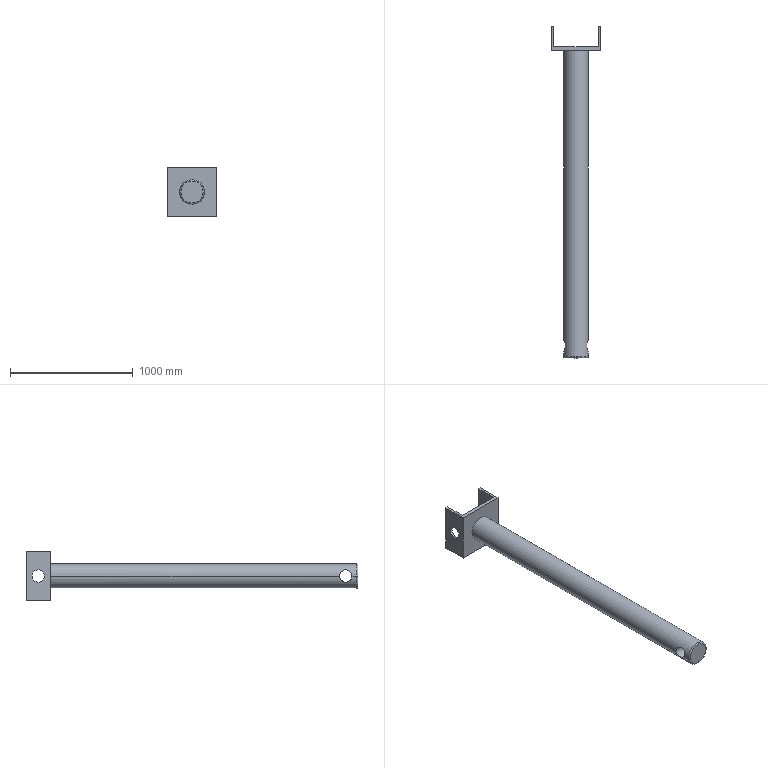Part | SolidWorks | features ICE 3, Extrusion 1, Fillet 1 | 1 solid | 21 faces | box 400 x 2700 x 400 mm | volume 84212442 mm3 | plane 11 | cylinder 8 | torus 2 | commonest cylinder face diameters 100 x6 200 x2
STEP:
#1=CARTESIAN_POINT('',(-100.,-2520.,200.));
#2=VERTEX_POINT('',#1);
#3=CARTESIAN_POINT('',(100.,-2520.,200.));
#4=VERTEX_POINT('',#3);
#5=CARTESIAN_POINT('',(0.,-2520.,200.));
#6=DIRECTION('',(0.,1.,0.));
#7=DIRECTION('',(1.,0.,0.));
#8=AXIS2_PLACEMENT_3D('',#5,#6,#7);
#9=CIRCLE('',#8,100.);
#10=EDGE_CURVE('',#2,#4,#9,.T.);
#11=ORIENTED_EDGE('',*,*,#10,.F.);
#12=CARTESIAN_POINT('',(-90.,-2530.,200.));
#13=VERTEX_POINT('',#12);
#14=CARTESIAN_POINT('',(-90.,-2520.,200.));
#15=DIRECTION('',(0.,0.,1.));
#16=DIRECTION('',(1.,0.,0.));
#17=AXIS2_PLACEMENT_3D('',#14,#15,#16);
#18=CIRCLE('',#17,10.);
#19=EDGE_CURVE('',#2,#13,#18,.T.);
#20=ORIENTED_EDGE('',*,*,#19,.T.);
#21=CARTESIAN_POINT('',(90.,-2530.,200.));
#22=VERTEX_POINT('',#21);
#23=CARTESIAN_POINT('',(0.,-2530.,200.));
#24=DIRECTION('',(0.,-1.,0.));
#25=DIRECTION('',(1.,0.,0.));
#26=AXIS2_PLACEMENT_3D('',#23,#24,#25);
#27=CIRCLE('',#26,90.);
#28=EDGE_CURVE('',#22,#13,#27,.T.);
#29=ORIENTED_EDGE('',*,*,#28,.F.);
#30=CARTESIAN_POINT('',(90.,-2520.,200.));
#31=DIRECTION('',(0.,0.,-1.));
#32=DIRECTION('',(-1.,0.,0.));
#33=AXIS2_PLACEMENT_3D('',#30,#31,#32);
#34=CIRCLE('',#33,10.);
#35=EDGE_CURVE('',#4,#22,#34,.T.);
#36=ORIENTED_EDGE('',*,*,#35,.F.);
#37=EDGE_LOOP('',(#11,#20,#29,#36));
#38=FACE_OUTER_BOUND('',#37,.T.);
#39=CARTESIAN_POINT('',(0.,-2520.,200.));
#40=DIRECTION('',(0.,-1.,0.));
#41=DIRECTION('',(1.,0.,0.));
#42=AXIS2_PLACEMENT_3D('',#39,#40,#41);
#43=TOROIDAL_SURFACE('',#42,90.,10.);
#44=ADVANCED_FACE('',(#38),#43,.T.);
#45=CARTESIAN_POINT('',(100.,-2480.,200.));
#46=VERTEX_POINT('',#45);
#47=CARTESIAN_POINT('',(86.603,-2430.,150.));
#48=VERTEX_POINT('',#47);
#49=CARTESIAN_POINT('',(100.,-2480.,200.));
#50=CARTESIAN_POINT('',(100.,-2480.,199.167));
#51=CARTESIAN_POINT('',(99.99,-2479.979,198.332));
#52=CARTESIAN_POINT('',(99.948,-2479.895,196.655));
#53=CARTESIAN_POINT('',(99.916,-2479.832,195.817));
#54=CARTESIAN_POINT('',(99.791,-2479.581,193.326));
#55=CARTESIAN_POINT('',(99.667,-2479.332,191.687));
#56=CARTESIAN_POINT('',(99.344,-2478.676,188.45));
#57=CARTESIAN_POINT('',(99.145,-2478.269,186.853));
#58=CARTESIAN_POINT('',(98.793,-2477.54,184.487));
#59=CARTESIAN_POINT('',(98.666,-2477.277,183.704));
#60=CARTESIAN_POINT('',(98.397,-2476.712,182.148));
#61=CARTESIAN_POINT('',(98.253,-2476.409,181.376));
#62=CARTESIAN_POINT('',(97.504,-2474.814,177.583));
#63=CARTESIAN_POINT('',(96.795,-2473.266,174.73));
#64=CARTESIAN_POINT('',(95.817,-2471.002,171.373));
#65=CARTESIAN_POINT('',(95.617,-2470.532,170.712));
#66=CARTESIAN_POINT('',(95.209,-2469.559,169.411));
#67=CARTESIAN_POINT('',(95.001,-2469.055,168.77));
#68=CARTESIAN_POINT('',(94.371,-2467.507,166.896));
#69=CARTESIAN_POINT('',(93.944,-2466.422,165.707));
#70=CARTESIAN_POINT('',(92.657,-2463.013,162.311));
#71=CARTESIAN_POINT('',(91.792,-2460.535,160.274));
#72=CARTESIAN_POINT('',(90.759,-2457.159,158.012));
#73=CARTESIAN_POINT('',(90.555,-2456.471,157.574));
#74=CARTESIAN_POINT('',(90.159,-2455.08,156.738));
#75=CARTESIAN_POINT('',(89.965,-2454.377,156.337));
#76=CARTESIAN_POINT('',(89.402,-2452.239,155.189));
#77=CARTESIAN_POINT('',(89.049,-2450.779,154.493));
#78=CARTESIAN_POINT('',(88.398,-2447.788,153.243));
#79=CARTESIAN_POINT('',(88.102,-2446.257,152.688));
#80=CARTESIAN_POINT('',(87.708,-2443.902,151.965));
#81=CARTESIAN_POINT('',(87.585,-2443.108,151.742));
#82=CARTESIAN_POINT('',(87.359,-2441.499,151.333));
#83=CARTESIAN_POINT('',(87.255,-2440.683,151.147));
#84=CARTESIAN_POINT('',(86.793,-2436.603,150.326));
#85=CARTESIAN_POINT('',(86.603,-2433.314,150.));
#86=CARTESIAN_POINT('',(86.603,-2430.,150.));
#87=B_SPLINE_CURVE_WITH_KNOTS('',3,(#49,#50,#51,#52,#53,#54,#55,#56,#57,#58,#59,#60,#61,#62,#63,#64,#65,#66,#67,#68,#69,#70,#71,#72,#73,#74,#75,#76,#77,#78,#79,#80,#81,#82,#83,#84,#85,#86),.UNSPECIFIED.,.F.,.F.,(4,2,2,2,2,2,2,2,2,2,2,2,2,2,2,2,2,2,4),(0.07955,0.08203,0.08452,0.08948,0.09445,0.09693,0.09942,0.1094,0.1118,0.1143,0.1193,0.1292,0.1317,0.1342,0.1392,0.1441,0.1466,0.1491,0.159),.UNSPECIFIED.);
#88=EDGE_CURVE('',#46,#48,#87,.T.);
#89=ORIENTED_EDGE('',*,*,#88,.T.);
#90=CARTESIAN_POINT('',(-86.603,-2430.,150.));
#91=VERTEX_POINT('',#90);
#92=CARTESIAN_POINT('',(2500.,-2430.,150.));
#93=DIRECTION('',(-1.,0.,0.));
#94=VECTOR('',#93,1000.);
#95=LINE('',#92,#94);
#96=EDGE_CURVE('',#48,#91,#95,.T.);
#97=ORIENTED_EDGE('',*,*,#96,.T.);
#98=CARTESIAN_POINT('',(-100.,-2480.,200.));
#99=VERTEX_POINT('',#98);
#100=CARTESIAN_POINT('',(-86.603,-2430.,150.));
#101=CARTESIAN_POINT('',(-86.603,-2431.652,150.));
#102=CARTESIAN_POINT('',(-86.65,-2433.306,150.082));
#103=CARTESIAN_POINT('',(-86.792,-2435.79,150.329));
#104=CARTESIAN_POINT('',(-86.851,-2436.618,150.433));
#105=CARTESIAN_POINT('',(-86.993,-2438.274,150.682));
#106=CARTESIAN_POINT('',(-87.075,-2439.095,150.827));
#107=CARTESIAN_POINT('',(-87.537,-2443.158,151.648));
#108=CARTESIAN_POINT('',(-88.072,-2446.288,152.614));
#109=CARTESIAN_POINT('',(-88.893,-2450.064,154.195));
#110=CARTESIAN_POINT('',(-89.066,-2450.813,154.53));
#111=CARTESIAN_POINT('',(-89.423,-2452.292,155.237));
#112=CARTESIAN_POINT('',(-89.607,-2453.019,155.607));
#113=CARTESIAN_POINT('',(-90.174,-2455.164,156.763));
#114=CARTESIAN_POINT('',(-90.571,-2456.545,157.598));
#115=CARTESIAN_POINT('',(-91.389,-2459.216,159.392));
#116=CARTESIAN_POINT('',(-91.811,-2460.506,160.352));
#117=CARTESIAN_POINT('',(-92.454,-2462.374,161.887));
#118=CARTESIAN_POINT('',(-92.67,-2462.985,162.415));
#119=CARTESIAN_POINT('',(-93.104,-2464.185,163.503));
#120=CARTESIAN_POINT('',(-93.321,-2464.771,164.061));
#121=CARTESIAN_POINT('',(-94.398,-2467.622,166.91));
#122=CARTESIAN_POINT('',(-95.238,-2469.661,169.382));
#123=CARTESIAN_POINT('',(-96.406,-2472.364,173.394));
#124=CARTESIAN_POINT('',(-96.779,-2473.205,174.781));
#125=CARTESIAN_POINT('',(-97.309,-2474.375,176.945));
#126=CARTESIAN_POINT('',(-97.48,-2474.748,177.677));
#127=CARTESIAN_POINT('',(-97.806,-2475.454,179.153));
#128=CARTESIAN_POINT('',(-97.962,-2475.789,179.899));
#129=CARTESIAN_POINT('',(-98.704,-2477.367,183.66));
#130=CARTESIAN_POINT('',(-99.176,-2478.335,186.782));
#131=CARTESIAN_POINT('',(-99.583,-2479.16,190.837));
#132=CARTESIAN_POINT('',(-99.655,-2479.306,191.655));
#133=CARTESIAN_POINT('',(-99.779,-2479.557,193.308));
#134=CARTESIAN_POINT('',(-99.832,-2479.663,194.142));
#135=CARTESIAN_POINT('',(-99.916,-2479.831,195.81));
#136=CARTESIAN_POINT('',(-99.947,-2479.894,196.645));
#137=CARTESIAN_POINT('',(-99.989,-2479.979,198.32));
#138=CARTESIAN_POINT('',(-100.,-2480.,199.161));
#139=CARTESIAN_POINT('',(-100.,-2480.,200.));
#140=B_SPLINE_CURVE_WITH_KNOTS('',3,(#100,#101,#102,#103,#104,#105,#106,#107,#108,#109,#110,#111,#112,#113,#114,#115,#116,#117,#118,#119,#120,#121,#122,#123,#124,#125,#126,#127,#128,#129,#130,#131,#132,#133,#134,#135,#136,#137,#138,#139),.UNSPECIFIED.,.F.,.F.,(4,2,2,2,2,2,2,2,2,2,2,2,2,2,2,2,2,2,2,4),(0.2385,0.2434,0.2459,0.2484,0.2583,0.2608,0.2633,0.2682,0.2732,0.2757,0.2782,0.2881,0.293,0.2955,0.298,0.3079,0.3104,0.3129,0.3153,0.3178),.UNSPECIFIED.);
#141=EDGE_CURVE('',#91,#99,#140,.T.);
#142=ORIENTED_EDGE('',*,*,#141,.T.);
#143=CARTESIAN_POINT('',(-86.603,-2430.,250.));
#144=VERTEX_POINT('',#143);
#145=CARTESIAN_POINT('',(-100.,-2480.,200.));
#146=CARTESIAN_POINT('',(-100.,-2480.,203.367));
#147=CARTESIAN_POINT('',(-99.831,-2479.663,206.667));
#148=CARTESIAN_POINT('',(-99.347,-2478.682,211.524));
#149=CARTESIAN_POINT('',(-99.148,-2478.275,213.128));
#150=CARTESIAN_POINT('',(-98.793,-2477.541,215.509));
#151=CARTESIAN_POINT('',(-98.666,-2477.276,216.298));
#152=CARTESIAN_POINT('',(-98.397,-2476.712,217.851));
#153=CARTESIAN_POINT('',(-98.255,-2476.412,218.617));
#154=CARTESIAN_POINT('',(-97.509,-2474.825,222.392));
#155=CARTESIAN_POINT('',(-96.801,-2473.28,225.247));
#156=CARTESIAN_POINT('',(-95.819,-2471.006,228.621));
#157=CARTESIAN_POINT('',(-95.618,-2470.533,229.287));
#158=CARTESIAN_POINT('',(-95.209,-2469.559,230.589));
#159=CARTESIAN_POINT('',(-95.002,-2469.059,231.226));
#160=CARTESIAN_POINT('',(-94.375,-2467.517,233.092));
#161=CARTESIAN_POINT('',(-93.949,-2466.435,234.279));
#162=CARTESIAN_POINT('',(-93.091,-2464.163,236.544));
#163=CARTESIAN_POINT('',(-92.66,-2462.973,237.622));
#164=CARTESIAN_POINT('',(-92.017,-2461.104,239.156));
#165=CARTESIAN_POINT('',(-91.803,-2460.467,239.654));
#166=CARTESIAN_POINT('',(-91.379,-2459.164,240.621));
#167=CARTESIAN_POINT('',(-91.169,-2458.499,241.091));
#168=CARTESIAN_POINT('',(-90.139,-2455.133,243.345));
#169=CARTESIAN_POINT('',(-89.378,-2452.293,244.873));
#170=CARTESIAN_POINT('',(-88.4,-2447.797,246.754));
#171=CARTESIAN_POINT('',(-88.102,-2446.258,247.312));
#172=CARTESIAN_POINT('',(-87.705,-2443.886,248.04));
#173=CARTESIAN_POINT('',(-87.581,-2443.082,248.265));
#174=CARTESIAN_POINT('',(-87.356,-2441.473,248.673));
#175=CARTESIAN_POINT('',(-87.253,-2440.665,248.856));
#176=CARTESIAN_POINT('',(-86.795,-2436.615,249.671));
#177=CARTESIAN_POINT('',(-86.603,-2433.33,250.));
#178=CARTESIAN_POINT('',(-86.603,-2430.,250.));
#179=B_SPLINE_CURVE_WITH_KNOTS('',3,(#145,#146,#147,#148,#149,#150,#151,#152,#153,#154,#155,#156,#157,#158,#159,#160,#161,#162,#163,#164,#165,#166,#167,#168,#169,#170,#171,#172,#173,#174,#175,#176,#177,#178),.UNSPECIFIED.,.F.,.F.,(4,2,2,2,2,2,2,2,2,2,2,2,2,2,2,2,4),(0.,0.009947,0.01492,0.01741,0.01989,0.02984,0.03233,0.03481,0.03979,0.04476,0.04725,0.04973,0.05968,0.06465,0.06714,0.06963,0.07957),.UNSPECIFIED.);
#180=EDGE_CURVE('',#99,#144,#179,.T.);
#181=ORIENTED_EDGE('',*,*,#180,.T.);
#182=CARTESIAN_POINT('',(86.603,-2430.,250.));
#183=VERTEX_POINT('',#182);
#184=CARTESIAN_POINT('',(2500.,-2430.,250.));
#185=DIRECTION('',(-1.,0.,0.));
#186=VECTOR('',#185,1000.);
#187=LINE('',#184,#186);
#188=EDGE_CURVE('',#183,#144,#187,.T.);
#189=ORIENTED_EDGE('',*,*,#188,.F.);
#190=CARTESIAN_POINT('',(86.603,-2430.,250.));
#191=CARTESIAN_POINT('',(86.603,-2433.368,250.));
#192=CARTESIAN_POINT('',(86.799,-2436.665,249.663));
#193=CARTESIAN_POINT('',(87.35,-2441.515,248.684));
#194=CARTESIAN_POINT('',(87.576,-2443.115,248.278));
#195=CARTESIAN_POINT('',(87.974,-2445.491,247.547));
#196=CARTESIAN_POINT('',(88.116,-2446.278,247.283));
#197=CARTESIAN_POINT('',(88.415,-2447.825,246.722));
#198=CARTESIAN_POINT('',(88.572,-2448.589,246.423));
#199=CARTESIAN_POINT('',(89.392,-2452.352,244.845));
#200=CARTESIAN_POINT('',(90.158,-2455.199,243.308));
#201=CARTESIAN_POINT('',(91.19,-2458.567,241.044));
#202=CARTESIAN_POINT('',(91.401,-2459.232,240.573));
#203=CARTESIAN_POINT('',(91.825,-2460.531,239.604));
#204=CARTESIAN_POINT('',(92.038,-2461.167,239.106));
#205=CARTESIAN_POINT('',(92.681,-2463.031,237.571));
#206=CARTESIAN_POINT('',(93.112,-2464.219,236.492));
#207=CARTESIAN_POINT('',(93.969,-2466.486,234.224));
#208=CARTESIAN_POINT('',(94.395,-2467.567,233.035));
#209=CARTESIAN_POINT('',(95.022,-2469.107,231.166));
#210=CARTESIAN_POINT('',(95.229,-2469.607,230.528));
#211=CARTESIAN_POINT('',(95.637,-2470.579,229.223));
#212=CARTESIAN_POINT('',(95.838,-2471.051,228.557));
#213=CARTESIAN_POINT('',(96.817,-2473.316,225.186));
#214=CARTESIAN_POINT('',(97.521,-2474.852,222.338));
#215=CARTESIAN_POINT('',(98.41,-2476.742,217.828));
#216=CARTESIAN_POINT('',(98.678,-2477.303,216.285));
#217=CARTESIAN_POINT('',(99.032,-2478.034,213.906));
#218=CARTESIAN_POINT('',(99.141,-2478.26,213.101));
#219=CARTESIAN_POINT('',(99.341,-2478.669,211.489));
#220=CARTESIAN_POINT('',(99.431,-2478.853,210.68));
#221=CARTESIAN_POINT('',(99.834,-2479.67,206.623));
#222=CARTESIAN_POINT('',(100.,-2480.,203.334));
#223=CARTESIAN_POINT('',(100.,-2480.,200.));
#224=B_SPLINE_CURVE_WITH_KNOTS('',3,(#190,#191,#192,#193,#194,#195,#196,#197,#198,#199,#200,#201,#202,#203,#204,#205,#206,#207,#208,#209,#210,#211,#212,#213,#214,#215,#216,#217,#218,#219,#220,#221,#222,#223),.UNSPECIFIED.,.F.,.F.,(4,2,2,2,2,2,2,2,2,2,2,2,2,2,2,2,4),(0.,0.009943,0.01492,0.0174,0.01989,0.02983,0.03232,0.0348,0.03977,0.04475,0.04723,0.04972,0.05966,0.06463,0.06712,0.0696,0.07955),.UNSPECIFIED.);
#225=EDGE_CURVE('',#183,#46,#224,.T.);
#226=ORIENTED_EDGE('',*,*,#225,.T.);
#227=EDGE_LOOP('',(#89,#97,#142,#181,#189,#226));
#228=FACE_OUTER_BOUND('',#227,.T.);
#229=CARTESIAN_POINT('',(2500.,-2430.,200.));
#230=DIRECTION('',(-1.,0.,0.));
#231=DIRECTION('',(0.,0.,1.));
#232=AXIS2_PLACEMENT_3D('',#229,#230,#231);
#233=CYLINDRICAL_SURFACE('',#232,50.);
#234=ADVANCED_FACE('',(#228),#233,.F.);
#235=CARTESIAN_POINT('',(-200.,20.,200.));
#236=VERTEX_POINT('',#235);
#237=CARTESIAN_POINT('',(-200.,120.,200.));
#238=VERTEX_POINT('',#237);
#239=CARTESIAN_POINT('',(-200.,70.,200.));
#240=DIRECTION('',(1.,0.,0.));
#241=DIRECTION('',(0.,1.,0.));
#242=AXIS2_PLACEMENT_3D('',#239,#240,#241);
#243=CIRCLE('',#242,50.);
#244=EDGE_CURVE('',#236,#238,#243,.T.);
#245=ORIENTED_EDGE('',*,*,#244,.F.);
#246=CARTESIAN_POINT('',(-180.,20.,200.));
#247=VERTEX_POINT('',#246);
#248=CARTESIAN_POINT('',(-200.,20.,200.));
#249=DIRECTION('',(1.,0.,0.));
#250=VECTOR('',#249,1000.);
#251=LINE('',#248,#250);
#252=EDGE_CURVE('',#236,#247,#251,.T.);
#253=ORIENTED_EDGE('',*,*,#252,.T.);
#254=CARTESIAN_POINT('',(-180.,120.,200.));
#255=VERTEX_POINT('',#254);
#256=CARTESIAN_POINT('',(-180.,70.,200.));
#257=DIRECTION('',(-1.,0.,0.));
#258=DIRECTION('',(0.,-1.,0.));
#259=AXIS2_PLACEMENT_3D('',#256,#257,#258);
#260=CIRCLE('',#259,50.);
#261=EDGE_CURVE('',#255,#247,#260,.T.);
#262=ORIENTED_EDGE('',*,*,#261,.F.);
#263=CARTESIAN_POINT('',(-200.,120.,200.));
#264=DIRECTION('',(1.,0.,0.));
#265=VECTOR('',#264,1000.);
#266=LINE('',#263,#265);
#267=EDGE_CURVE('',#238,#255,#266,.T.);
#268=ORIENTED_EDGE('',*,*,#267,.F.);
#269=EDGE_LOOP('',(#245,#253,#262,#268));
#270=FACE_OUTER_BOUND('',#269,.T.);
#271=CARTESIAN_POINT('',(-200.,70.,200.));
#272=DIRECTION('',(1.,0.,0.));
#273=DIRECTION('',(0.,1.,0.));
#274=AXIS2_PLACEMENT_3D('',#271,#272,#273);
#275=CYLINDRICAL_SURFACE('',#274,50.);
#276=ADVANCED_FACE('',(#270),#275,.F.);
#277=CARTESIAN_POINT('',(180.,20.,200.));
#278=VERTEX_POINT('',#277);
#279=CARTESIAN_POINT('',(180.,120.,200.));
#280=VERTEX_POINT('',#279);
#281=CARTESIAN_POINT('',(180.,70.,200.));
#282=DIRECTION('',(1.,0.,0.));
#283=DIRECTION('',(0.,0.,-1.));
#284=AXIS2_PLACEMENT_3D('',#281,#282,#283);
#285=CIRCLE('',#284,50.);
#286=EDGE_CURVE('',#278,#280,#285,.T.);
#287=ORIENTED_EDGE('',*,*,#286,.F.);
#288=CARTESIAN_POINT('',(200.,20.,200.));
#289=VERTEX_POINT('',#288);
#290=CARTESIAN_POINT('',(-200.,20.,200.));
#291=DIRECTION('',(1.,0.,0.));
#292=VECTOR('',#291,1000.);
#293=LINE('',#290,#292);
#294=EDGE_CURVE('',#278,#289,#293,.T.);
#295=ORIENTED_EDGE('',*,*,#294,.T.);
#296=CARTESIAN_POINT('',(200.,120.,200.));
#297=VERTEX_POINT('',#296);
#298=CARTESIAN_POINT('',(200.,70.,200.));
#299=DIRECTION('',(1.,0.,0.));
#300=DIRECTION('',(0.,1.,0.));
#301=AXIS2_PLACEMENT_3D('',#298,#299,#300);
#302=CIRCLE('',#301,50.);
#303=EDGE_CURVE('',#289,#297,#302,.T.);
#304=ORIENTED_EDGE('',*,*,#303,.T.);
#305=CARTESIAN_POINT('',(-200.,120.,200.));
#306=DIRECTION('',(1.,0.,0.));
#307=VECTOR('',#306,1000.);
#308=LINE('',#305,#307);
#309=EDGE_CURVE('',#280,#297,#308,.T.);
#310=ORIENTED_EDGE('',*,*,#309,.F.);
#311=EDGE_LOOP('',(#287,#295,#304,#310));
#312=FACE_OUTER_BOUND('',#311,.T.);
#313=CARTESIAN_POINT('',(-200.,70.,200.));
#314=DIRECTION('',(1.,0.,0.));
#315=DIRECTION('',(0.,1.,0.));
#316=AXIS2_PLACEMENT_3D('',#313,#314,#315);
#317=CYLINDRICAL_SURFACE('',#316,50.);
#318=ADVANCED_FACE('',(#312),#317,.F.);
#319=ORIENTED_EDGE('',*,*,#10,.T.);
#320=CARTESIAN_POINT('',(100.,-2530.,200.));
#321=DIRECTION('',(0.,1.,0.));
#322=VECTOR('',#321,1000.);
#323=LINE('',#320,#322);
#324=EDGE_CURVE('',#4,#46,#323,.T.);
#325=ORIENTED_EDGE('',*,*,#324,.T.);
#326=ORIENTED_EDGE('',*,*,#225,.F.);
#327=CARTESIAN_POINT('',(100.,-2380.,200.));
#328=VERTEX_POINT('',#327);
#329=CARTESIAN_POINT('',(100.,-2380.,200.));
#330=CARTESIAN_POINT('',(100.,-2380.,201.654));
#331=CARTESIAN_POINT('',(99.959,-2380.082,203.31));
#332=CARTESIAN_POINT('',(99.835,-2380.33,205.797));
#333=CARTESIAN_POINT('',(99.784,-2380.434,206.628));
#334=CARTESIAN_POINT('',(99.66,-2380.684,208.284));
#335=CARTESIAN_POINT('',(99.588,-2380.829,209.104));
#336=CARTESIAN_POINT('',(99.183,-2381.652,213.17));
#337=CARTESIAN_POINT('',(98.71,-2382.62,216.308));
#338=CARTESIAN_POINT('',(97.964,-2384.208,220.093));
#339=CARTESIAN_POINT('',(97.806,-2384.545,220.844));
#340=CARTESIAN_POINT('',(97.478,-2385.255,222.329));
#341=CARTESIAN_POINT('',(97.308,-2385.627,223.059));
#342=CARTESIAN_POINT('',(96.781,-2386.79,225.211));
#343=CARTESIAN_POINT('',(96.408,-2387.63,226.596));
#344=CARTESIAN_POINT('',(95.63,-2389.432,229.272));
#345=CARTESIAN_POINT('',(95.224,-2390.396,230.563));
#346=CARTESIAN_POINT('',(94.598,-2391.935,232.43));
#347=CARTESIAN_POINT('',(94.386,-2392.464,233.041));
#348=CARTESIAN_POINT('',(93.958,-2393.554,234.24));
#349=CARTESIAN_POINT('',(93.741,-2394.115,234.827));
#350=CARTESIAN_POINT('',(92.663,-2396.97,237.676));
#351=CARTESIAN_POINT('',(91.8,-2399.444,239.707));
#352=CARTESIAN_POINT('',(90.573,-2403.448,242.398));
#353=CARTESIAN_POINT('',(90.175,-2404.832,243.235));
#354=CARTESIAN_POINT('',(89.605,-2406.988,244.397));
#355=CARTESIAN_POINT('',(89.42,-2407.718,244.768));
#356=CARTESIAN_POINT('',(89.065,-2409.19,245.471));
#357=CARTESIAN_POINT('',(88.894,-2409.932,245.803));
#358=CARTESIAN_POINT('',(88.078,-2413.681,247.374));
#359=CARTESIAN_POINT('',(87.545,-2416.794,248.337));
#360=CARTESIAN_POINT('',(87.082,-2420.839,249.161));
#361=CARTESIAN_POINT('',(87.,-2421.656,249.306));
#362=CARTESIAN_POINT('',(86.857,-2423.306,249.557));
#363=CARTESIAN_POINT('',(86.797,-2424.14,249.663));
#364=CARTESIAN_POINT('',(86.7,-2425.808,249.831));
#365=CARTESIAN_POINT('',(86.663,-2426.644,249.894));
#366=CARTESIAN_POINT('',(86.615,-2428.319,249.979));
#367=CARTESIAN_POINT('',(86.603,-2429.16,250.));
#368=CARTESIAN_POINT('',(86.603,-2430.,250.));
#369=B_SPLINE_CURVE_WITH_KNOTS('',3,(#329,#330,#331,#332,#333,#334,#335,#336,#337,#338,#339,#340,#341,#342,#343,#344,#345,#346,#347,#348,#349,#350,#351,#352,#353,#354,#355,#356,#357,#358,#359,#360,#361,#362,#363,#364,#365,#366,#367,#368),.UNSPECIFIED.,.F.,.F.,(4,2,2,2,2,2,2,2,2,2,2,2,2,2,2,2,2,2,2,4),(0.2384,0.2434,0.2459,0.2484,0.2583,0.2608,0.2632,0.2682,0.2732,0.2756,0.2781,0.288,0.293,0.2955,0.2979,0.3079,0.3103,0.3128,0.3153,0.3178),.UNSPECIFIED.);
#370=EDGE_CURVE('',#328,#183,#369,.T.);
#371=ORIENTED_EDGE('',*,*,#370,.F.);
#372=CARTESIAN_POINT('',(100.,-30.,200.));
#373=VERTEX_POINT('',#372);
#374=CARTESIAN_POINT('',(100.,-2530.,200.));
#375=DIRECTION('',(0.,1.,0.));
#376=VECTOR('',#375,1000.);
#377=LINE('',#374,#376);
#378=EDGE_CURVE('',#328,#373,#377,.T.);
#379=ORIENTED_EDGE('',*,*,#378,.T.);
#380=CARTESIAN_POINT('',(-100.,-30.,200.));
#381=VERTEX_POINT('',#380);
#382=CARTESIAN_POINT('',(0.,-30.,200.));
#383=DIRECTION('',(0.,-1.,0.));
#384=DIRECTION('',(-1.,0.,0.));
#385=AXIS2_PLACEMENT_3D('',#382,#383,#384);
#386=CIRCLE('',#385,100.);
#387=EDGE_CURVE('',#373,#381,#386,.T.);
#388=ORIENTED_EDGE('',*,*,#387,.T.);
#389=CARTESIAN_POINT('',(-100.,-2380.,200.));
#390=VERTEX_POINT('',#389);
#391=CARTESIAN_POINT('',(-100.,-2530.,200.));
#392=DIRECTION('',(0.,1.,0.));
#393=VECTOR('',#392,1000.);
#394=LINE('',#391,#393);
#395=EDGE_CURVE('',#390,#381,#394,.T.);
#396=ORIENTED_EDGE('',*,*,#395,.F.);
#397=CARTESIAN_POINT('',(-86.603,-2430.,250.));
#398=CARTESIAN_POINT('',(-86.603,-2429.168,250.));
#399=CARTESIAN_POINT('',(-86.615,-2428.334,249.979));
#400=CARTESIAN_POINT('',(-86.663,-2426.66,249.895));
#401=CARTESIAN_POINT('',(-86.699,-2425.82,249.832));
#402=CARTESIAN_POINT('',(-86.843,-2423.328,249.581));
#403=CARTESIAN_POINT('',(-86.986,-2421.689,249.332));
#404=CARTESIAN_POINT('',(-87.354,-2418.457,248.677));
#405=CARTESIAN_POINT('',(-87.58,-2416.862,248.271));
#406=CARTESIAN_POINT('',(-87.975,-2414.502,247.545));
#407=CARTESIAN_POINT('',(-88.116,-2413.721,247.283));
#408=CARTESIAN_POINT('',(-88.416,-2412.169,246.72));
#409=CARTESIAN_POINT('',(-88.574,-2411.4,246.419));
#410=CARTESIAN_POINT('',(-89.399,-2407.621,244.832));
#411=CARTESIAN_POINT('',(-90.165,-2404.776,243.292));
#412=CARTESIAN_POINT('',(-91.193,-2401.424,241.037));
#413=CARTESIAN_POINT('',(-91.402,-2400.764,240.57));
#414=CARTESIAN_POINT('',(-91.826,-2399.464,239.6));
#415=CARTESIAN_POINT('',(-92.041,-2398.824,239.099));
#416=CARTESIAN_POINT('',(-92.686,-2396.953,237.557));
#417=CARTESIAN_POINT('',(-93.118,-2395.765,236.476));
#418=CARTESIAN_POINT('',(-94.403,-2392.365,233.074));
#419=CARTESIAN_POINT('',(-95.246,-2390.32,230.596));
#420=CARTESIAN_POINT('',(-96.229,-2388.046,227.212));
#421=CARTESIAN_POINT('',(-96.421,-2387.606,226.523));
#422=CARTESIAN_POINT('',(-96.794,-2386.766,225.129));
#423=CARTESIAN_POINT('',(-96.974,-2386.363,224.423));
#424=CARTESIAN_POINT('',(-97.498,-2385.209,222.28));
#425=CARTESIAN_POINT('',(-97.822,-2384.51,220.816));
#426=CARTESIAN_POINT('',(-98.412,-2383.253,217.815));
#427=CARTESIAN_POINT('',(-98.679,-2382.696,216.279));
#428=CARTESIAN_POINT('',(-99.03,-2381.969,213.919));
#429=CARTESIAN_POINT('',(-99.139,-2381.745,213.122));
#430=CARTESIAN_POINT('',(-99.339,-2381.336,211.51));
#431=CARTESIAN_POINT('',(-99.43,-2381.15,210.692));
#432=CARTESIAN_POINT('',(-99.835,-2380.327,206.61));
#433=CARTESIAN_POINT('',(-100.,-2380.,203.318));
#434=CARTESIAN_POINT('',(-100.,-2380.,200.));
#435=B_SPLINE_CURVE_WITH_KNOTS('',3,(#397,#398,#399,#400,#401,#402,#403,#404,#405,#406,#407,#408,#409,#410,#411,#412,#413,#414,#415,#416,#417,#418,#419,#420,#421,#422,#423,#424,#425,#426,#427,#428,#429,#430,#431,#432,#433,#434),.UNSPECIFIED.,.F.,.F.,(4,2,2,2,2,2,2,2,2,2,2,2,2,2,2,2,2,2,4),(0.07957,0.08206,0.08454,0.08951,0.09447,0.09696,0.09944,0.1094,0.1119,0.1143,0.1193,0.1292,0.1317,0.1342,0.1392,0.1441,0.1466,0.1491,0.159),.UNSPECIFIED.);
#436=EDGE_CURVE('',#144,#390,#435,.T.);
#437=ORIENTED_EDGE('',*,*,#436,.F.);
#438=ORIENTED_EDGE('',*,*,#180,.F.);
#439=CARTESIAN_POINT('',(-100.,-2530.,200.));
#440=DIRECTION('',(0.,1.,0.));
#441=VECTOR('',#440,1000.);
#442=LINE('',#439,#441);
#443=EDGE_CURVE('',#2,#99,#442,.T.);
#444=ORIENTED_EDGE('',*,*,#443,.F.);
#445=EDGE_LOOP('',(#319,#325,#326,#371,#379,#388,#396,#437,#438,#444));
#446=FACE_OUTER_BOUND('',#445,.T.);
#447=CARTESIAN_POINT('',(0.,-2530.,200.));
#448=DIRECTION('',(0.,1.,0.));
#449=DIRECTION('',(-1.,0.,0.));
#450=AXIS2_PLACEMENT_3D('',#447,#448,#449);
#451=CYLINDRICAL_SURFACE('',#450,100.);
#452=ADVANCED_FACE('',(#446),#451,.T.);
#453=ORIENTED_EDGE('',*,*,#324,.F.);
#454=CARTESIAN_POINT('',(0.,-2520.,200.));
#455=DIRECTION('',(0.,1.,0.));
#456=DIRECTION('',(1.,0.,0.));
#457=AXIS2_PLACEMENT_3D('',#454,#455,#456);
#458=CIRCLE('',#457,100.);
#459=EDGE_CURVE('',#4,#2,#458,.T.);
#460=ORIENTED_EDGE('',*,*,#459,.T.);
#461=ORIENTED_EDGE('',*,*,#443,.T.);
#462=ORIENTED_EDGE('',*,*,#141,.F.);
#463=CARTESIAN_POINT('',(-100.,-2380.,200.));
#464=CARTESIAN_POINT('',(-100.,-2380.,198.342));
#465=CARTESIAN_POINT('',(-99.959,-2380.082,196.677));
#466=CARTESIAN_POINT('',(-99.792,-2380.418,193.334));
#467=CARTESIAN_POINT('',(-99.667,-2380.668,191.688));
#468=CARTESIAN_POINT('',(-99.182,-2381.654,186.824));
#469=CARTESIAN_POINT('',(-98.708,-2382.623,183.681));
#470=CARTESIAN_POINT('',(-97.956,-2384.223,179.872));
#471=CARTESIAN_POINT('',(-97.799,-2384.561,179.12));
#472=CARTESIAN_POINT('',(-97.472,-2385.269,177.643));
#473=CARTESIAN_POINT('',(-97.302,-2385.64,176.916));
#474=CARTESIAN_POINT('',(-96.776,-2386.801,174.771));
#475=CARTESIAN_POINT('',(-96.404,-2387.64,173.387));
#476=CARTESIAN_POINT('',(-95.624,-2389.447,170.707));
#477=CARTESIAN_POINT('',(-95.216,-2390.414,169.412));
#478=CARTESIAN_POINT('',(-94.586,-2391.964,167.536));
#479=CARTESIAN_POINT('',(-94.373,-2392.497,166.921));
#480=CARTESIAN_POINT('',(-93.945,-2393.586,165.726));
#481=CARTESIAN_POINT('',(-93.731,-2394.143,165.144));
#482=CARTESIAN_POINT('',(-92.656,-2396.99,162.308));
#483=CARTESIAN_POINT('',(-91.792,-2399.465,160.275));
#484=CARTESIAN_POINT('',(-90.765,-2402.82,158.025));
#485=CARTESIAN_POINT('',(-90.563,-2403.504,157.59));
#486=CARTESIAN_POINT('',(-90.164,-2404.9,156.749));
#487=CARTESIAN_POINT('',(-89.969,-2405.61,156.345));
#488=CARTESIAN_POINT('',(-89.402,-2407.759,155.19));
#489=CARTESIAN_POINT('',(-89.048,-2409.223,154.492));
#490=CARTESIAN_POINT('',(-88.073,-2413.712,152.616));
#491=CARTESIAN_POINT('',(-87.538,-2416.832,151.65));
#492=CARTESIAN_POINT('',(-87.074,-2420.913,150.826));
#493=CARTESIAN_POINT('',(-86.992,-2421.74,150.68));
#494=CARTESIAN_POINT('',(-86.851,-2423.39,150.432));
#495=CARTESIAN_POINT('',(-86.792,-2424.215,150.329));
#496=CARTESIAN_POINT('',(-86.65,-2426.692,150.082));
#497=CARTESIAN_POINT('',(-86.603,-2428.345,150.));
#498=CARTESIAN_POINT('',(-86.603,-2430.,150.));
#499=B_SPLINE_CURVE_WITH_KNOTS('',3,(#463,#464,#465,#466,#467,#468,#469,#470,#471,#472,#473,#474,#475,#476,#477,#478,#479,#480,#481,#482,#483,#484,#485,#486,#487,#488,#489,#490,#491,#492,#493,#494,#495,#496,#497,#498),.UNSPECIFIED.,.F.,.F.,(4,2,2,2,2,2,2,2,2,2,2,2,2,2,2,2,2,4),(0.159,0.164,0.169,0.1789,0.1814,0.1839,0.1888,0.1938,0.1963,0.1988,0.2087,0.2112,0.2137,0.2186,0.2286,0.231,0.2335,0.2385),.UNSPECIFIED.);
#500=EDGE_CURVE('',#390,#91,#499,.T.);
#501=ORIENTED_EDGE('',*,*,#500,.F.);
#502=ORIENTED_EDGE('',*,*,#395,.T.);
#503=CARTESIAN_POINT('',(0.,-30.,200.));
#504=DIRECTION('',(0.,-1.,0.));
#505=DIRECTION('',(-1.,0.,0.));
#506=AXIS2_PLACEMENT_3D('',#503,#504,#505);
#507=CIRCLE('',#506,100.);
#508=EDGE_CURVE('',#381,#373,#507,.T.);
#509=ORIENTED_EDGE('',*,*,#508,.T.);
#510=ORIENTED_EDGE('',*,*,#378,.F.);
#511=CARTESIAN_POINT('',(86.603,-2430.,150.));
#512=CARTESIAN_POINT('',(86.603,-2428.344,150.));
#513=CARTESIAN_POINT('',(86.65,-2426.682,150.082));
#514=CARTESIAN_POINT('',(86.794,-2424.179,150.333));
#515=CARTESIAN_POINT('',(86.854,-2423.347,150.438));
#516=CARTESIAN_POINT('',(86.995,-2421.701,150.687));
#517=CARTESIAN_POINT('',(87.077,-2420.884,150.831));
#518=CARTESIAN_POINT('',(87.538,-2416.835,151.651));
#519=CARTESIAN_POINT('',(88.073,-2413.699,152.617));
#520=CARTESIAN_POINT('',(89.067,-2409.142,154.529));
#521=CARTESIAN_POINT('',(89.425,-2407.669,155.234));
#522=CARTESIAN_POINT('',(90.179,-2404.817,156.774));
#523=CARTESIAN_POINT('',(90.576,-2403.437,157.609));
#524=CARTESIAN_POINT('',(91.396,-2400.762,159.408));
#525=CARTESIAN_POINT('',(91.82,-2399.468,160.372));
#526=CARTESIAN_POINT('',(92.466,-2397.591,161.917));
#527=CARTESIAN_POINT('',(92.683,-2396.977,162.448));
#528=CARTESIAN_POINT('',(93.116,-2395.783,163.533));
#529=CARTESIAN_POINT('',(93.331,-2395.2,164.089));
#530=CARTESIAN_POINT('',(94.405,-2392.362,166.929));
#531=CARTESIAN_POINT('',(95.245,-2390.322,169.403));
#532=CARTESIAN_POINT('',(96.222,-2388.061,172.765));
#533=CARTESIAN_POINT('',(96.414,-2387.623,173.451));
#534=CARTESIAN_POINT('',(96.789,-2386.777,174.851));
#535=CARTESIAN_POINT('',(96.971,-2386.371,175.563));
#536=CARTESIAN_POINT('',(97.497,-2385.209,177.719));
#537=CARTESIAN_POINT('',(97.822,-2384.508,179.187));
#538=CARTESIAN_POINT('',(98.709,-2382.623,183.691));
#539=CARTESIAN_POINT('',(99.182,-2381.653,186.821));
#540=CARTESIAN_POINT('',(99.589,-2380.826,190.909));
#541=CARTESIAN_POINT('',(99.661,-2380.68,191.737));
#542=CARTESIAN_POINT('',(99.785,-2380.432,193.387));
#543=CARTESIAN_POINT('',(99.836,-2380.329,194.212));
#544=CARTESIAN_POINT('',(99.959,-2380.082,196.69));
#545=CARTESIAN_POINT('',(100.,-2380.,198.344));
#546=CARTESIAN_POINT('',(100.,-2380.,200.));
#547=B_SPLINE_CURVE_WITH_KNOTS('',3,(#511,#512,#513,#514,#515,#516,#517,#518,#519,#520,#521,#522,#523,#524,#525,#526,#527,#528,#529,#530,#531,#532,#533,#534,#535,#536,#537,#538,#539,#540,#541,#542,#543,#544,#545,#546),.UNSPECIFIED.,.F.,.F.,(4,2,2,2,2,2,2,2,2,2,2,2,2,2,2,2,2,4),(0.159,0.164,0.1665,0.169,0.1789,0.1838,0.1888,0.1938,0.1963,0.1987,0.2087,0.2111,0.2136,0.2186,0.2285,0.231,0.2335,0.2384),.UNSPECIFIED.);
#548=EDGE_CURVE('',#48,#328,#547,.T.);
#549=ORIENTED_EDGE('',*,*,#548,.F.);
#550=ORIENTED_EDGE('',*,*,#88,.F.);
#551=EDGE_LOOP('',(#453,#460,#461,#462,#501,#502,#509,#510,#549,#550));
#552=FACE_OUTER_BOUND('',#551,.T.);
#553=CARTESIAN_POINT('',(0.,-2530.,200.));
#554=DIRECTION('',(0.,1.,0.));
#555=DIRECTION('',(-1.,0.,0.));
#556=AXIS2_PLACEMENT_3D('',#553,#554,#555);
#557=CYLINDRICAL_SURFACE('',#556,100.);
#558=ADVANCED_FACE('',(#552),#557,.T.);
#559=CARTESIAN_POINT('',(-200.,-30.,0.));
#560=VERTEX_POINT('',#559);
#561=CARTESIAN_POINT('',(200.,-30.,0.));
#562=VERTEX_POINT('',#561);
#563=CARTESIAN_POINT('',(200.,-30.,0.));
#564=DIRECTION('',(1.,0.,0.));
#565=VECTOR('',#564,1000.);
#566=LINE('',#563,#565);
#567=EDGE_CURVE('',#560,#562,#566,.T.);
#568=ORIENTED_EDGE('',*,*,#567,.T.);
#569=CARTESIAN_POINT('',(200.,-30.,400.));
#570=VERTEX_POINT('',#569);
#571=CARTESIAN_POINT('',(200.,-30.,400.));
#572=DIRECTION('',(0.,0.,-1.));
#573=VECTOR('',#572,1000.);
#574=LINE('',#571,#573);
#575=EDGE_CURVE('',#570,#562,#574,.T.);
#576=ORIENTED_EDGE('',*,*,#575,.F.);
#577=CARTESIAN_POINT('',(-200.,-30.,400.));
#578=VERTEX_POINT('',#577);
#579=CARTESIAN_POINT('',(200.,-30.,400.));
#580=DIRECTION('',(1.,0.,0.));
#581=VECTOR('',#580,1000.);
#582=LINE('',#579,#581);
#583=EDGE_CURVE('',#578,#570,#582,.T.);
#584=ORIENTED_EDGE('',*,*,#583,.F.);
#585=CARTESIAN_POINT('',(-200.,-30.,400.));
#586=DIRECTION('',(0.,0.,-1.));
#587=VECTOR('',#586,1000.);
#588=LINE('',#585,#587);
#589=EDGE_CURVE('',#578,#560,#588,.T.);
#590=ORIENTED_EDGE('',*,*,#589,.T.);
#591=EDGE_LOOP('',(#568,#576,#584,#590));
#592=FACE_OUTER_BOUND('',#591,.T.);
#593=ORIENTED_EDGE('',*,*,#508,.F.);
#594=ORIENTED_EDGE('',*,*,#387,.F.);
#595=EDGE_LOOP('',(#593,#594));
#596=FACE_BOUND('',#595,.T.);
#597=CARTESIAN_POINT('',(200.,-30.,400.));
#598=DIRECTION('',(0.,1.,0.));
#599=DIRECTION('',(-1.,0.,0.));
#600=AXIS2_PLACEMENT_3D('',#597,#598,#599);
#601=PLANE('',#600);
#602=ADVANCED_FACE('',(#592,#596),#601,.F.);
#603=ORIENTED_EDGE('',*,*,#261,.T.);
#604=CARTESIAN_POINT('',(-180.,70.,200.));
#605=DIRECTION('',(-1.,0.,0.));
#606=DIRECTION('',(0.,-1.,0.));
#607=AXIS2_PLACEMENT_3D('',#604,#605,#606);
#608=CIRCLE('',#607,50.);
#609=EDGE_CURVE('',#247,#255,#608,.T.);
#610=ORIENTED_EDGE('',*,*,#609,.T.);
#611=EDGE_LOOP('',(#603,#610));
#612=FACE_BOUND('',#611,.T.);
#613=CARTESIAN_POINT('',(-180.,0.,0.));
#614=VERTEX_POINT('',#613);
#615=CARTESIAN_POINT('',(-180.,170.,0.));
#616=VERTEX_POINT('',#615);
#617=CARTESIAN_POINT('',(-180.,170.,0.));
#618=DIRECTION('',(0.,1.,0.));
#619=VECTOR('',#618,1000.);
#620=LINE('',#617,#619);
#621=EDGE_CURVE('',#614,#616,#620,.T.);
#622=ORIENTED_EDGE('',*,*,#621,.T.);
#623=CARTESIAN_POINT('',(-180.,170.,400.));
#624=VERTEX_POINT('',#623);
#625=CARTESIAN_POINT('',(-180.,170.,400.));
#626=DIRECTION('',(0.,0.,-1.));
#627=VECTOR('',#626,1000.);
#628=LINE('',#625,#627);
#629=EDGE_CURVE('',#624,#616,#628,.T.);
#630=ORIENTED_EDGE('',*,*,#629,.F.);
#631=CARTESIAN_POINT('',(-180.,0.,400.));
#632=VERTEX_POINT('',#631);
#633=CARTESIAN_POINT('',(-180.,170.,400.));
#634=DIRECTION('',(0.,1.,0.));
#635=VECTOR('',#634,1000.);
#636=LINE('',#633,#635);
#637=EDGE_CURVE('',#632,#624,#636,.T.);
#638=ORIENTED_EDGE('',*,*,#637,.F.);
#639=CARTESIAN_POINT('',(-180.,0.,400.));
#640=DIRECTION('',(0.,0.,-1.));
#641=VECTOR('',#640,1000.);
#642=LINE('',#639,#641);
#643=EDGE_CURVE('',#632,#614,#642,.T.);
#644=ORIENTED_EDGE('',*,*,#643,.T.);
#645=EDGE_LOOP('',(#622,#630,#638,#644));
#646=FACE_OUTER_BOUND('',#645,.T.);
#647=CARTESIAN_POINT('',(-180.,170.,400.));
#648=DIRECTION('',(-1.,0.,0.));
#649=DIRECTION('',(0.,-1.,0.));
#650=AXIS2_PLACEMENT_3D('',#647,#648,#649);
#651=PLANE('',#650);
#652=ADVANCED_FACE('',(#612,#646),#651,.F.);
#653=CARTESIAN_POINT('',(-200.,170.,0.));
#654=VERTEX_POINT('',#653);
#655=CARTESIAN_POINT('',(-200.,170.,0.));
#656=DIRECTION('',(-1.,0.,0.));
#657=VECTOR('',#656,1000.);
#658=LINE('',#655,#657);
#659=EDGE_CURVE('',#616,#654,#658,.T.);
#660=ORIENTED_EDGE('',*,*,#659,.T.);
#661=CARTESIAN_POINT('',(-200.,170.,400.));
#662=VERTEX_POINT('',#661);
#663=CARTESIAN_POINT('',(-200.,170.,400.));
#664=DIRECTION('',(0.,0.,-1.));
#665=VECTOR('',#664,1000.);
#666=LINE('',#663,#665);
#667=EDGE_CURVE('',#662,#654,#666,.T.);
#668=ORIENTED_EDGE('',*,*,#667,.F.);
#669=CARTESIAN_POINT('',(-200.,170.,400.));
#670=DIRECTION('',(-1.,0.,0.));
#671=VECTOR('',#670,1000.);
#672=LINE('',#669,#671);
#673=EDGE_CURVE('',#624,#662,#672,.T.);
#674=ORIENTED_EDGE('',*,*,#673,.F.);
#675=ORIENTED_EDGE('',*,*,#629,.T.);
#676=EDGE_LOOP('',(#660,#668,#674,#675));
#677=FACE_OUTER_BOUND('',#676,.T.);
#678=CARTESIAN_POINT('',(-200.,170.,400.));
#679=DIRECTION('',(0.,-1.,0.));
#680=DIRECTION('',(0.,0.,-1.));
#681=AXIS2_PLACEMENT_3D('',#678,#679,#680);
#682=PLANE('',#681);
#683=ADVANCED_FACE('',(#677),#682,.F.);
#684=CARTESIAN_POINT('',(-200.,70.,200.));
#685=DIRECTION('',(1.,0.,0.));
#686=DIRECTION('',(0.,1.,0.));
#687=AXIS2_PLACEMENT_3D('',#684,#685,#686);
#688=CIRCLE('',#687,50.);
#689=EDGE_CURVE('',#238,#236,#688,.T.);
#690=ORIENTED_EDGE('',*,*,#689,.T.);
#691=ORIENTED_EDGE('',*,*,#244,.T.);
#692=EDGE_LOOP('',(#690,#691));
#693=FACE_BOUND('',#692,.T.);
#694=CARTESIAN_POINT('',(-200.,-30.,0.));
#695=DIRECTION('',(0.,-1.,0.));
#696=VECTOR('',#695,1000.);
#697=LINE('',#694,#696);
#698=EDGE_CURVE('',#654,#560,#697,.T.);
#699=ORIENTED_EDGE('',*,*,#698,.T.);
#700=ORIENTED_EDGE('',*,*,#589,.F.);
#701=CARTESIAN_POINT('',(-200.,-30.,400.));
#702=DIRECTION('',(0.,-1.,0.));
#703=VECTOR('',#702,1000.);
#704=LINE('',#701,#703);
#705=EDGE_CURVE('',#662,#578,#704,.T.);
#706=ORIENTED_EDGE('',*,*,#705,.F.);
#707=ORIENTED_EDGE('',*,*,#667,.T.);
#708=EDGE_LOOP('',(#699,#700,#706,#707));
#709=FACE_OUTER_BOUND('',#708,.T.);
#710=CARTESIAN_POINT('',(-200.,-30.,400.));
#711=DIRECTION('',(1.,0.,0.));
#712=DIRECTION('',(0.,1.,0.));
#713=AXIS2_PLACEMENT_3D('',#710,#711,#712);
#714=PLANE('',#713);
#715=ADVANCED_FACE('',(#693,#709),#714,.F.);
#716=CARTESIAN_POINT('',(200.,70.,200.));
#717=DIRECTION('',(1.,0.,0.));
#718=DIRECTION('',(0.,1.,0.));
#719=AXIS2_PLACEMENT_3D('',#716,#717,#718);
#720=CIRCLE('',#719,50.);
#721=EDGE_CURVE('',#297,#289,#720,.T.);
#722=ORIENTED_EDGE('',*,*,#721,.F.);
#723=ORIENTED_EDGE('',*,*,#303,.F.);
#724=EDGE_LOOP('',(#722,#723));
#725=FACE_BOUND('',#724,.T.);
#726=CARTESIAN_POINT('',(200.,170.,0.));
#727=VERTEX_POINT('',#726);
#728=CARTESIAN_POINT('',(200.,170.,0.));
#729=DIRECTION('',(0.,1.,0.));
#730=VECTOR('',#729,1000.);
#731=LINE('',#728,#730);
#732=EDGE_CURVE('',#562,#727,#731,.T.);
#733=ORIENTED_EDGE('',*,*,#732,.T.);
#734=CARTESIAN_POINT('',(200.,170.,400.));
#735=VERTEX_POINT('',#734);
#736=CARTESIAN_POINT('',(200.,170.,400.));
#737=DIRECTION('',(0.,0.,-1.));
#738=VECTOR('',#737,1000.);
#739=LINE('',#736,#738);
#740=EDGE_CURVE('',#735,#727,#739,.T.);
#741=ORIENTED_EDGE('',*,*,#740,.F.);
#742=CARTESIAN_POINT('',(200.,170.,400.));
#743=DIRECTION('',(0.,1.,0.));
#744=VECTOR('',#743,1000.);
#745=LINE('',#742,#744);
#746=EDGE_CURVE('',#570,#735,#745,.T.);
#747=ORIENTED_EDGE('',*,*,#746,.F.);
#748=ORIENTED_EDGE('',*,*,#575,.T.);
#749=EDGE_LOOP('',(#733,#741,#747,#748));
#750=FACE_OUTER_BOUND('',#749,.T.);
#751=CARTESIAN_POINT('',(200.,170.,400.));
#752=DIRECTION('',(-1.,0.,0.));
#753=DIRECTION('',(0.,-1.,0.));
#754=AXIS2_PLACEMENT_3D('',#751,#752,#753);
#755=PLANE('',#754);
#756=ADVANCED_FACE('',(#725,#750),#755,.F.);
#757=CARTESIAN_POINT('',(180.,170.,0.));
#758=VERTEX_POINT('',#757);
#759=CARTESIAN_POINT('',(180.,170.,0.));
#760=DIRECTION('',(-1.,0.,0.));
#761=VECTOR('',#760,1000.);
#762=LINE('',#759,#761);
#763=EDGE_CURVE('',#727,#758,#762,.T.);
#764=ORIENTED_EDGE('',*,*,#763,.T.);
#765=CARTESIAN_POINT('',(180.,170.,400.));
#766=VERTEX_POINT('',#765);
#767=CARTESIAN_POINT('',(180.,170.,400.));
#768=DIRECTION('',(0.,0.,-1.));
#769=VECTOR('',#768,1000.);
#770=LINE('',#767,#769);
#771=EDGE_CURVE('',#766,#758,#770,.T.);
#772=ORIENTED_EDGE('',*,*,#771,.F.);
#773=CARTESIAN_POINT('',(180.,170.,400.));
#774=DIRECTION('',(-1.,0.,0.));
#775=VECTOR('',#774,1000.);
#776=LINE('',#773,#775);
#777=EDGE_CURVE('',#735,#766,#776,.T.);
#778=ORIENTED_EDGE('',*,*,#777,.F.);
#779=ORIENTED_EDGE('',*,*,#740,.T.);
#780=EDGE_LOOP('',(#764,#772,#778,#779));
#781=FACE_OUTER_BOUND('',#780,.T.);
#782=CARTESIAN_POINT('',(180.,170.,400.));
#783=DIRECTION('',(0.,-1.,0.));
#784=DIRECTION('',(0.,0.,-1.));
#785=AXIS2_PLACEMENT_3D('',#782,#783,#784);
#786=PLANE('',#785);
#787=ADVANCED_FACE('',(#781),#786,.F.);
#788=CARTESIAN_POINT('',(180.,70.,200.));
#789=DIRECTION('',(1.,0.,0.));
#790=DIRECTION('',(0.,0.,-1.));
#791=AXIS2_PLACEMENT_3D('',#788,#789,#790);
#792=CIRCLE('',#791,50.);
#793=EDGE_CURVE('',#280,#278,#792,.T.);
#794=ORIENTED_EDGE('',*,*,#793,.T.);
#795=ORIENTED_EDGE('',*,*,#286,.T.);
#796=EDGE_LOOP('',(#794,#795));
#797=FACE_BOUND('',#796,.T.);
#798=CARTESIAN_POINT('',(180.,0.,0.));
#799=VERTEX_POINT('',#798);
#800=CARTESIAN_POINT('',(180.,0.,0.));
#801=DIRECTION('',(0.,-1.,0.));
#802=VECTOR('',#801,1000.);
#803=LINE('',#800,#802);
#804=EDGE_CURVE('',#758,#799,#803,.T.);
#805=ORIENTED_EDGE('',*,*,#804,.T.);
#806=CARTESIAN_POINT('',(180.,0.,400.));
#807=VERTEX_POINT('',#806);
#808=CARTESIAN_POINT('',(180.,0.,400.));
#809=DIRECTION('',(0.,0.,-1.));
#810=VECTOR('',#809,1000.);
#811=LINE('',#808,#810);
#812=EDGE_CURVE('',#807,#799,#811,.T.);
#813=ORIENTED_EDGE('',*,*,#812,.F.);
#814=CARTESIAN_POINT('',(180.,0.,400.));
#815=DIRECTION('',(0.,-1.,0.));
#816=VECTOR('',#815,1000.);
#817=LINE('',#814,#816);
#818=EDGE_CURVE('',#766,#807,#817,.T.);
#819=ORIENTED_EDGE('',*,*,#818,.F.);
#820=ORIENTED_EDGE('',*,*,#771,.T.);
#821=EDGE_LOOP('',(#805,#813,#819,#820));
#822=FACE_OUTER_BOUND('',#821,.T.);
#823=CARTESIAN_POINT('',(180.,0.,400.));
#824=DIRECTION('',(1.,0.,0.));
#825=DIRECTION('',(0.,0.,-1.));
#826=AXIS2_PLACEMENT_3D('',#823,#824,#825);
#827=PLANE('',#826);
#828=ADVANCED_FACE('',(#797,#822),#827,.F.);
#829=CARTESIAN_POINT('',(-180.,0.,0.));
#830=DIRECTION('',(-1.,0.,0.));
#831=VECTOR('',#830,1000.);
#832=LINE('',#829,#831);
#833=EDGE_CURVE('',#799,#614,#832,.T.);
#834=ORIENTED_EDGE('',*,*,#833,.T.);
#835=ORIENTED_EDGE('',*,*,#643,.F.);
#836=CARTESIAN_POINT('',(-180.,0.,400.));
#837=DIRECTION('',(-1.,0.,0.));
#838=VECTOR('',#837,1000.);
#839=LINE('',#836,#838);
#840=EDGE_CURVE('',#807,#632,#839,.T.);
#841=ORIENTED_EDGE('',*,*,#840,.F.);
#842=ORIENTED_EDGE('',*,*,#812,.T.);
#843=EDGE_LOOP('',(#834,#835,#841,#842));
#844=FACE_OUTER_BOUND('',#843,.T.);
#845=CARTESIAN_POINT('',(-180.,0.,400.));
#846=DIRECTION('',(0.,-1.,0.));
#847=DIRECTION('',(0.,0.,-1.));
#848=AXIS2_PLACEMENT_3D('',#845,#846,#847);
#849=PLANE('',#848);
#850=ADVANCED_FACE('',(#844),#849,.F.);
#851=ORIENTED_EDGE('',*,*,#637,.T.);
#852=ORIENTED_EDGE('',*,*,#673,.T.);
#853=ORIENTED_EDGE('',*,*,#705,.T.);
#854=ORIENTED_EDGE('',*,*,#583,.T.);
#855=ORIENTED_EDGE('',*,*,#746,.T.);
#856=ORIENTED_EDGE('',*,*,#777,.T.);
#857=ORIENTED_EDGE('',*,*,#818,.T.);
#858=ORIENTED_EDGE('',*,*,#840,.T.);
#859=EDGE_LOOP('',(#851,#852,#853,#854,#855,#856,#857,#858));
#860=FACE_OUTER_BOUND('',#859,.T.);
#861=CARTESIAN_POINT('',(-180.,0.,400.));
#862=DIRECTION('',(0.,0.,1.));
#863=DIRECTION('',(1.,0.,0.));
#864=AXIS2_PLACEMENT_3D('',#861,#862,#863);
#865=PLANE('',#864);
#866=ADVANCED_FACE('',(#860),#865,.T.);
#867=ORIENTED_EDGE('',*,*,#621,.F.);
#868=ORIENTED_EDGE('',*,*,#833,.F.);
#869=ORIENTED_EDGE('',*,*,#804,.F.);
#870=ORIENTED_EDGE('',*,*,#763,.F.);
#871=ORIENTED_EDGE('',*,*,#732,.F.);
#872=ORIENTED_EDGE('',*,*,#567,.F.);
#873=ORIENTED_EDGE('',*,*,#698,.F.);
#874=ORIENTED_EDGE('',*,*,#659,.F.);
#875=EDGE_LOOP('',(#867,#868,#869,#870,#871,#872,#873,#874));
#876=FACE_OUTER_BOUND('',#875,.T.);
#877=CARTESIAN_POINT('',(-180.,0.,0.));
#878=DIRECTION('',(0.,0.,1.));
#879=DIRECTION('',(1.,0.,0.));
#880=AXIS2_PLACEMENT_3D('',#877,#878,#879);
#881=PLANE('',#880);
#882=ADVANCED_FACE('',(#876),#881,.F.);
#883=ORIENTED_EDGE('',*,*,#294,.F.);
#884=ORIENTED_EDGE('',*,*,#793,.F.);
#885=ORIENTED_EDGE('',*,*,#309,.T.);
#886=ORIENTED_EDGE('',*,*,#721,.T.);
#887=EDGE_LOOP('',(#883,#884,#885,#886));
#888=FACE_OUTER_BOUND('',#887,.T.);
#889=CARTESIAN_POINT('',(-200.,70.,200.));
#890=DIRECTION('',(1.,0.,0.));
#891=DIRECTION('',(0.,1.,0.));
#892=AXIS2_PLACEMENT_3D('',#889,#890,#891);
#893=CYLINDRICAL_SURFACE('',#892,50.);
#894=ADVANCED_FACE('',(#888),#893,.F.);
#895=ORIENTED_EDGE('',*,*,#252,.F.);
#896=ORIENTED_EDGE('',*,*,#689,.F.);
#897=ORIENTED_EDGE('',*,*,#267,.T.);
#898=ORIENTED_EDGE('',*,*,#609,.F.);
#899=EDGE_LOOP('',(#895,#896,#897,#898));
#900=FACE_OUTER_BOUND('',#899,.T.);
#901=CARTESIAN_POINT('',(-200.,70.,200.));
#902=DIRECTION('',(1.,0.,0.));
#903=DIRECTION('',(0.,1.,0.));
#904=AXIS2_PLACEMENT_3D('',#901,#902,#903);
#905=CYLINDRICAL_SURFACE('',#904,50.);
#906=ADVANCED_FACE('',(#900),#905,.F.);
#907=ORIENTED_EDGE('',*,*,#28,.T.);
#908=CARTESIAN_POINT('',(0.,-2530.,200.));
#909=DIRECTION('',(0.,-1.,0.));
#910=DIRECTION('',(1.,0.,0.));
#911=AXIS2_PLACEMENT_3D('',#908,#909,#910);
#912=CIRCLE('',#911,90.);
#913=EDGE_CURVE('',#13,#22,#912,.T.);
#914=ORIENTED_EDGE('',*,*,#913,.T.);
#915=EDGE_LOOP('',(#907,#914));
#916=FACE_OUTER_BOUND('',#915,.T.);
#917=CARTESIAN_POINT('',(0.,-2530.,200.));
#918=DIRECTION('',(0.,-1.,0.));
#919=DIRECTION('',(1.,0.,0.));
#920=AXIS2_PLACEMENT_3D('',#917,#918,#919);
#921=PLANE('',#920);
#922=ADVANCED_FACE('',(#916),#921,.T.);
#923=ORIENTED_EDGE('',*,*,#96,.F.);
#924=ORIENTED_EDGE('',*,*,#548,.T.);
#925=ORIENTED_EDGE('',*,*,#370,.T.);
#926=ORIENTED_EDGE('',*,*,#188,.T.);
#927=ORIENTED_EDGE('',*,*,#436,.T.);
#928=ORIENTED_EDGE('',*,*,#500,.T.);
#929=EDGE_LOOP('',(#923,#924,#925,#926,#927,#928));
#930=FACE_OUTER_BOUND('',#929,.T.);
#931=CARTESIAN_POINT('',(2500.,-2430.,200.));
#932=DIRECTION('',(-1.,0.,0.));
#933=DIRECTION('',(0.,0.,1.));
#934=AXIS2_PLACEMENT_3D('',#931,#932,#933);
#935=CYLINDRICAL_SURFACE('',#934,50.);
#936=ADVANCED_FACE('',(#930),#935,.F.);
#937=ORIENTED_EDGE('',*,*,#19,.F.);
#938=ORIENTED_EDGE('',*,*,#459,.F.);
#939=ORIENTED_EDGE('',*,*,#35,.T.);
#940=ORIENTED_EDGE('',*,*,#913,.F.);
#941=EDGE_LOOP('',(#937,#938,#939,#940));
#942=FACE_OUTER_BOUND('',#941,.T.);
#943=CARTESIAN_POINT('',(0.,-2520.,200.));
#944=DIRECTION('',(0.,-1.,0.));
#945=DIRECTION('',(1.,0.,0.));
#946=AXIS2_PLACEMENT_3D('',#943,#944,#945);
#947=TOROIDAL_SURFACE('',#946,90.,10.);
#948=ADVANCED_FACE('',(#942),#947,.T.);
#949=CLOSED_SHELL('',(#44,#234,#276,#318,#452,#558,#602,#652,#683,#715,#756,#787,#828,#850,#866,#882,#894,#906,#922,#936,#948));
#950=MANIFOLD_SOLID_BREP('',#949);
#951=CARTESIAN_POINT('',(0.,0.,0.));
#952=DIRECTION('',(0.,0.,1.));
#953=DIRECTION('',(1.,0.,0.));
#954=AXIS2_PLACEMENT_3D('',#951,#952,#953);
#955=(LENGTH_UNIT()NAMED_UNIT(*)SI_UNIT(.MILLI.,.METRE.));
#956=UNCERTAINTY_MEASURE_WITH_UNIT(LENGTH_MEASURE(0.00001),#955,'','');
#957=(NAMED_UNIT(*)PLANE_ANGLE_UNIT()SI_UNIT($,.RADIAN.));
#958=(NAMED_UNIT(*)SI_UNIT($,.STERADIAN.)SOLID_ANGLE_UNIT());
#959=(GEOMETRIC_REPRESENTATION_CONTEXT(3)GLOBAL_UNCERTAINTY_ASSIGNED_CONTEXT((#956))GLOBAL_UNIT_ASSIGNED_CONTEXT((#955,#957,#958))REPRESENTATION_CONTEXT('',''));
#960=ADVANCED_BREP_SHAPE_REPRESENTATION('',(#950,#954),#959);